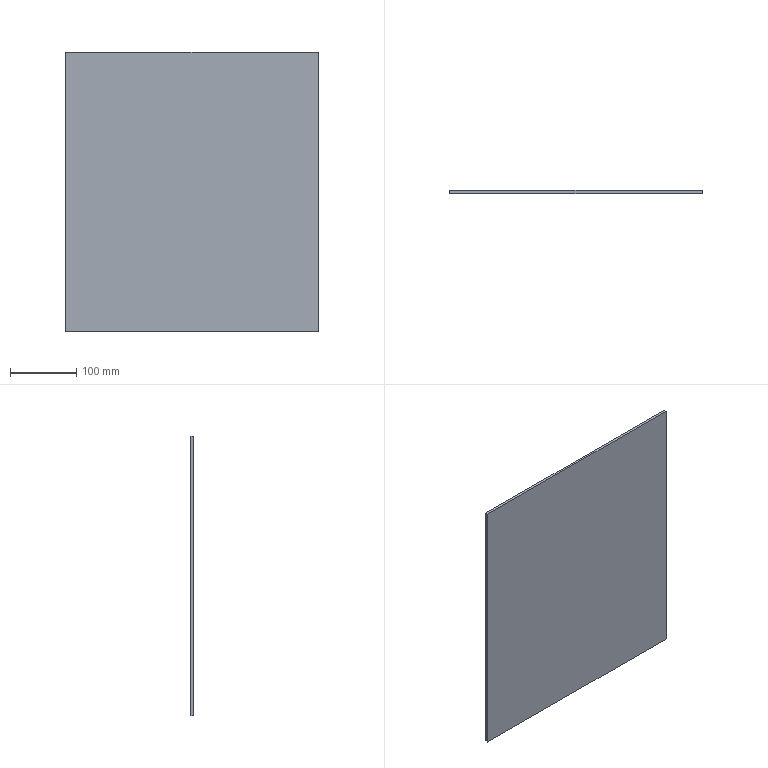Part | SolidWorks | features Extrusion 1, ICE 1 | 1 solid | 6 faces | box 380 x 4 x 420 mm | volume 638400 mm3 | plane 6
STEP:
#1=CARTESIAN_POINT('',(190.,0.,210.));
#2=VERTEX_POINT('',#1);
#3=CARTESIAN_POINT('',(190.,0.,-210.));
#4=VERTEX_POINT('',#3);
#5=CARTESIAN_POINT('',(190.,0.,-210.));
#6=DIRECTION('',(0.,0.,-1.));
#7=VECTOR('',#6,1000.);
#8=LINE('',#5,#7);
#9=EDGE_CURVE('',#2,#4,#8,.T.);
#10=ORIENTED_EDGE('',*,*,#9,.T.);
#11=CARTESIAN_POINT('',(190.,4.,-210.));
#12=VERTEX_POINT('',#11);
#13=CARTESIAN_POINT('',(190.,4.,-210.));
#14=DIRECTION('',(0.,-1.,0.));
#15=VECTOR('',#14,1000.);
#16=LINE('',#13,#15);
#17=EDGE_CURVE('',#12,#4,#16,.T.);
#18=ORIENTED_EDGE('',*,*,#17,.F.);
#19=CARTESIAN_POINT('',(190.,4.,210.));
#20=VERTEX_POINT('',#19);
#21=CARTESIAN_POINT('',(190.,4.,-210.));
#22=DIRECTION('',(0.,0.,-1.));
#23=VECTOR('',#22,1000.);
#24=LINE('',#21,#23);
#25=EDGE_CURVE('',#20,#12,#24,.T.);
#26=ORIENTED_EDGE('',*,*,#25,.F.);
#27=CARTESIAN_POINT('',(190.,4.,210.));
#28=DIRECTION('',(0.,-1.,0.));
#29=VECTOR('',#28,1000.);
#30=LINE('',#27,#29);
#31=EDGE_CURVE('',#20,#2,#30,.T.);
#32=ORIENTED_EDGE('',*,*,#31,.T.);
#33=EDGE_LOOP('',(#10,#18,#26,#32));
#34=FACE_OUTER_BOUND('',#33,.T.);
#35=CARTESIAN_POINT('',(190.,4.,-210.));
#36=DIRECTION('',(-1.,0.,0.));
#37=DIRECTION('',(0.,0.,1.));
#38=AXIS2_PLACEMENT_3D('',#35,#36,#37);
#39=PLANE('',#38);
#40=ADVANCED_FACE('',(#34),#39,.F.);
#41=CARTESIAN_POINT('',(-190.,0.,-210.));
#42=VERTEX_POINT('',#41);
#43=CARTESIAN_POINT('',(-190.,0.,-210.));
#44=DIRECTION('',(-1.,0.,0.));
#45=VECTOR('',#44,1000.);
#46=LINE('',#43,#45);
#47=EDGE_CURVE('',#4,#42,#46,.T.);
#48=ORIENTED_EDGE('',*,*,#47,.T.);
#49=CARTESIAN_POINT('',(-190.,4.,-210.));
#50=VERTEX_POINT('',#49);
#51=CARTESIAN_POINT('',(-190.,4.,-210.));
#52=DIRECTION('',(0.,-1.,0.));
#53=VECTOR('',#52,1000.);
#54=LINE('',#51,#53);
#55=EDGE_CURVE('',#50,#42,#54,.T.);
#56=ORIENTED_EDGE('',*,*,#55,.F.);
#57=CARTESIAN_POINT('',(-190.,4.,-210.));
#58=DIRECTION('',(-1.,0.,0.));
#59=VECTOR('',#58,1000.);
#60=LINE('',#57,#59);
#61=EDGE_CURVE('',#12,#50,#60,.T.);
#62=ORIENTED_EDGE('',*,*,#61,.F.);
#63=ORIENTED_EDGE('',*,*,#17,.T.);
#64=EDGE_LOOP('',(#48,#56,#62,#63));
#65=FACE_OUTER_BOUND('',#64,.T.);
#66=CARTESIAN_POINT('',(-190.,4.,-210.));
#67=DIRECTION('',(0.,0.,1.));
#68=DIRECTION('',(1.,0.,0.));
#69=AXIS2_PLACEMENT_3D('',#66,#67,#68);
#70=PLANE('',#69);
#71=ADVANCED_FACE('',(#65),#70,.F.);
#72=CARTESIAN_POINT('',(-190.,0.,210.));
#73=VERTEX_POINT('',#72);
#74=CARTESIAN_POINT('',(-190.,0.,-210.));
#75=DIRECTION('',(0.,0.,1.));
#76=VECTOR('',#75,1000.);
#77=LINE('',#74,#76);
#78=EDGE_CURVE('',#42,#73,#77,.T.);
#79=ORIENTED_EDGE('',*,*,#78,.T.);
#80=CARTESIAN_POINT('',(-190.,4.,210.));
#81=VERTEX_POINT('',#80);
#82=CARTESIAN_POINT('',(-190.,4.,210.));
#83=DIRECTION('',(0.,-1.,0.));
#84=VECTOR('',#83,1000.);
#85=LINE('',#82,#84);
#86=EDGE_CURVE('',#81,#73,#85,.T.);
#87=ORIENTED_EDGE('',*,*,#86,.F.);
#88=CARTESIAN_POINT('',(-190.,4.,-210.));
#89=DIRECTION('',(0.,0.,1.));
#90=VECTOR('',#89,1000.);
#91=LINE('',#88,#90);
#92=EDGE_CURVE('',#50,#81,#91,.T.);
#93=ORIENTED_EDGE('',*,*,#92,.F.);
#94=ORIENTED_EDGE('',*,*,#55,.T.);
#95=EDGE_LOOP('',(#79,#87,#93,#94));
#96=FACE_OUTER_BOUND('',#95,.T.);
#97=CARTESIAN_POINT('',(-190.,4.,-210.));
#98=DIRECTION('',(1.,0.,0.));
#99=DIRECTION('',(0.,0.,-1.));
#100=AXIS2_PLACEMENT_3D('',#97,#98,#99);
#101=PLANE('',#100);
#102=ADVANCED_FACE('',(#96),#101,.F.);
#103=CARTESIAN_POINT('',(-190.,0.,210.));
#104=DIRECTION('',(1.,0.,0.));
#105=VECTOR('',#104,1000.);
#106=LINE('',#103,#105);
#107=EDGE_CURVE('',#73,#2,#106,.T.);
#108=ORIENTED_EDGE('',*,*,#107,.T.);
#109=ORIENTED_EDGE('',*,*,#31,.F.);
#110=CARTESIAN_POINT('',(-190.,4.,210.));
#111=DIRECTION('',(1.,0.,0.));
#112=VECTOR('',#111,1000.);
#113=LINE('',#110,#112);
#114=EDGE_CURVE('',#81,#20,#113,.T.);
#115=ORIENTED_EDGE('',*,*,#114,.F.);
#116=ORIENTED_EDGE('',*,*,#86,.T.);
#117=EDGE_LOOP('',(#108,#109,#115,#116));
#118=FACE_OUTER_BOUND('',#117,.T.);
#119=CARTESIAN_POINT('',(-190.,4.,210.));
#120=DIRECTION('',(0.,0.,-1.));
#121=DIRECTION('',(-1.,0.,0.));
#122=AXIS2_PLACEMENT_3D('',#119,#120,#121);
#123=PLANE('',#122);
#124=ADVANCED_FACE('',(#118),#123,.F.);
#125=ORIENTED_EDGE('',*,*,#25,.T.);
#126=ORIENTED_EDGE('',*,*,#61,.T.);
#127=ORIENTED_EDGE('',*,*,#92,.T.);
#128=ORIENTED_EDGE('',*,*,#114,.T.);
#129=EDGE_LOOP('',(#125,#126,#127,#128));
#130=FACE_OUTER_BOUND('',#129,.T.);
#131=CARTESIAN_POINT('',(0.,4.,0.));
#132=DIRECTION('',(0.,1.,0.));
#133=DIRECTION('',(0.,0.,1.));
#134=AXIS2_PLACEMENT_3D('',#131,#132,#133);
#135=PLANE('',#134);
#136=ADVANCED_FACE('',(#130),#135,.T.);
#137=ORIENTED_EDGE('',*,*,#9,.F.);
#138=ORIENTED_EDGE('',*,*,#107,.F.);
#139=ORIENTED_EDGE('',*,*,#78,.F.);
#140=ORIENTED_EDGE('',*,*,#47,.F.);
#141=EDGE_LOOP('',(#137,#138,#139,#140));
#142=FACE_OUTER_BOUND('',#141,.T.);
#143=CARTESIAN_POINT('',(0.,0.,0.));
#144=DIRECTION('',(0.,1.,0.));
#145=DIRECTION('',(0.,0.,1.));
#146=AXIS2_PLACEMENT_3D('',#143,#144,#145);
#147=PLANE('',#146);
#148=ADVANCED_FACE('',(#142),#147,.F.);
#149=CLOSED_SHELL('',(#40,#71,#102,#124,#136,#148));
#150=MANIFOLD_SOLID_BREP('',#149);
#151=CARTESIAN_POINT('',(0.,0.,0.));
#152=DIRECTION('',(0.,0.,1.));
#153=DIRECTION('',(1.,0.,0.));
#154=AXIS2_PLACEMENT_3D('',#151,#152,#153);
#155=(LENGTH_UNIT()NAMED_UNIT(*)SI_UNIT(.MILLI.,.METRE.));
#156=UNCERTAINTY_MEASURE_WITH_UNIT(LENGTH_MEASURE(0.00001),#155,'','');
#157=(NAMED_UNIT(*)PLANE_ANGLE_UNIT()SI_UNIT($,.RADIAN.));
#158=(NAMED_UNIT(*)SI_UNIT($,.STERADIAN.)SOLID_ANGLE_UNIT());
#159=(GEOMETRIC_REPRESENTATION_CONTEXT(3)GLOBAL_UNCERTAINTY_ASSIGNED_CONTEXT((#156))GLOBAL_UNIT_ASSIGNED_CONTEXT((#155,#157,#158))REPRESENTATION_CONTEXT('',''));
#160=ADVANCED_BREP_SHAPE_REPRESENTATION('',(#150,#154),#159);